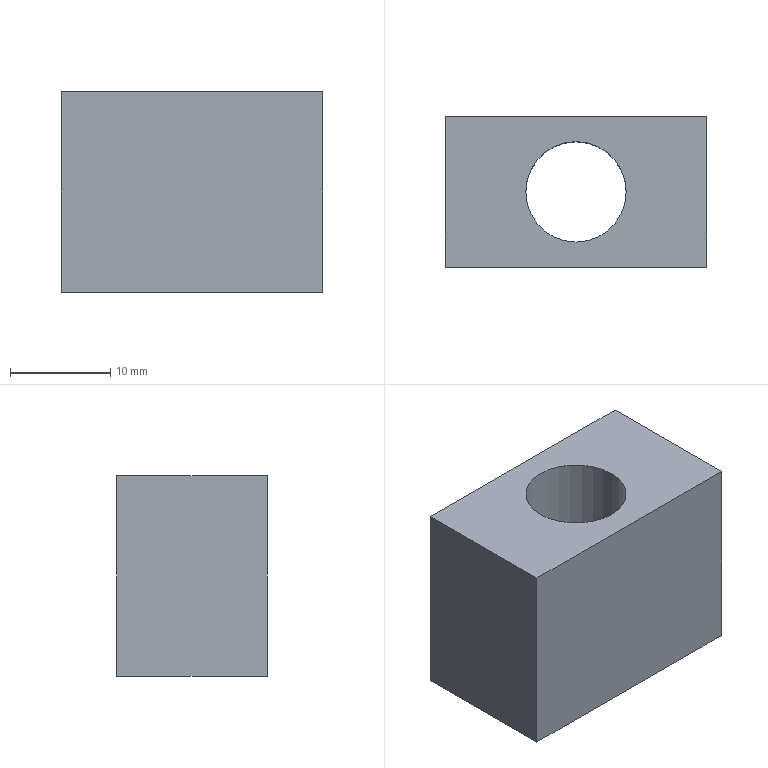Part | SolidWorks | features Extrusion 1 | 1 solid | 8 faces | box 26 x 15 x 20 mm | volume 6229 mm3 | plane 6 | cylinder 2 | commonest cylinder face diameters 10 x2
STEP:
#1=CARTESIAN_POINT('',(-5.,0.,20.));
#2=VERTEX_POINT('',#1);
#3=CARTESIAN_POINT('',(5.,0.,20.));
#4=VERTEX_POINT('',#3);
#5=CARTESIAN_POINT('',(0.,0.,20.));
#6=DIRECTION('',(0.,0.,1.));
#7=DIRECTION('',(1.,0.,0.));
#8=AXIS2_PLACEMENT_3D('',#5,#6,#7);
#9=CIRCLE('',#8,5.);
#10=EDGE_CURVE('',#2,#4,#9,.T.);
#11=ORIENTED_EDGE('',*,*,#10,.T.);
#12=CARTESIAN_POINT('',(5.,0.,0.));
#13=VERTEX_POINT('',#12);
#14=CARTESIAN_POINT('',(5.,0.,20.));
#15=DIRECTION('',(0.,0.,-1.));
#16=VECTOR('',#15,1000.);
#17=LINE('',#14,#16);
#18=EDGE_CURVE('',#4,#13,#17,.T.);
#19=ORIENTED_EDGE('',*,*,#18,.T.);
#20=CARTESIAN_POINT('',(-5.,0.,0.));
#21=VERTEX_POINT('',#20);
#22=CARTESIAN_POINT('',(0.,0.,0.));
#23=DIRECTION('',(0.,0.,1.));
#24=DIRECTION('',(1.,0.,0.));
#25=AXIS2_PLACEMENT_3D('',#22,#23,#24);
#26=CIRCLE('',#25,5.);
#27=EDGE_CURVE('',#21,#13,#26,.T.);
#28=ORIENTED_EDGE('',*,*,#27,.F.);
#29=CARTESIAN_POINT('',(-5.,0.,20.));
#30=DIRECTION('',(0.,0.,-1.));
#31=VECTOR('',#30,1000.);
#32=LINE('',#29,#31);
#33=EDGE_CURVE('',#2,#21,#32,.T.);
#34=ORIENTED_EDGE('',*,*,#33,.F.);
#35=EDGE_LOOP('',(#11,#19,#28,#34));
#36=FACE_OUTER_BOUND('',#35,.T.);
#37=CARTESIAN_POINT('',(0.,0.,20.));
#38=DIRECTION('',(0.,0.,-1.));
#39=DIRECTION('',(-1.,0.,0.));
#40=AXIS2_PLACEMENT_3D('',#37,#38,#39);
#41=CYLINDRICAL_SURFACE('',#40,5.);
#42=ADVANCED_FACE('',(#36),#41,.F.);
#43=CARTESIAN_POINT('',(13.,-7.5,20.));
#44=VERTEX_POINT('',#43);
#45=CARTESIAN_POINT('',(13.,7.5,20.));
#46=VERTEX_POINT('',#45);
#47=CARTESIAN_POINT('',(13.,7.5,20.));
#48=DIRECTION('',(0.,1.,0.));
#49=VECTOR('',#48,1000.);
#50=LINE('',#47,#49);
#51=EDGE_CURVE('',#44,#46,#50,.T.);
#52=ORIENTED_EDGE('',*,*,#51,.T.);
#53=CARTESIAN_POINT('',(-13.,7.5,20.));
#54=VERTEX_POINT('',#53);
#55=CARTESIAN_POINT('',(-13.,7.5,20.));
#56=DIRECTION('',(-1.,0.,0.));
#57=VECTOR('',#56,1000.);
#58=LINE('',#55,#57);
#59=EDGE_CURVE('',#46,#54,#58,.T.);
#60=ORIENTED_EDGE('',*,*,#59,.T.);
#61=CARTESIAN_POINT('',(-13.,-7.5,20.));
#62=VERTEX_POINT('',#61);
#63=CARTESIAN_POINT('',(-13.,7.5,20.));
#64=DIRECTION('',(0.,-1.,0.));
#65=VECTOR('',#64,1000.);
#66=LINE('',#63,#65);
#67=EDGE_CURVE('',#54,#62,#66,.T.);
#68=ORIENTED_EDGE('',*,*,#67,.T.);
#69=CARTESIAN_POINT('',(-13.,-7.5,20.));
#70=DIRECTION('',(1.,0.,0.));
#71=VECTOR('',#70,1000.);
#72=LINE('',#69,#71);
#73=EDGE_CURVE('',#62,#44,#72,.T.);
#74=ORIENTED_EDGE('',*,*,#73,.T.);
#75=EDGE_LOOP('',(#52,#60,#68,#74));
#76=FACE_OUTER_BOUND('',#75,.T.);
#77=ORIENTED_EDGE('',*,*,#10,.F.);
#78=CARTESIAN_POINT('',(0.,0.,20.));
#79=DIRECTION('',(0.,0.,1.));
#80=DIRECTION('',(1.,0.,0.));
#81=AXIS2_PLACEMENT_3D('',#78,#79,#80);
#82=CIRCLE('',#81,5.);
#83=EDGE_CURVE('',#4,#2,#82,.T.);
#84=ORIENTED_EDGE('',*,*,#83,.F.);
#85=EDGE_LOOP('',(#77,#84));
#86=FACE_BOUND('',#85,.T.);
#87=CARTESIAN_POINT('',(0.,0.,20.));
#88=DIRECTION('',(0.,0.,1.));
#89=DIRECTION('',(1.,0.,0.));
#90=AXIS2_PLACEMENT_3D('',#87,#88,#89);
#91=PLANE('',#90);
#92=ADVANCED_FACE('',(#76,#86),#91,.T.);
#93=CARTESIAN_POINT('',(13.,-7.5,0.));
#94=VERTEX_POINT('',#93);
#95=CARTESIAN_POINT('',(13.,7.5,0.));
#96=VERTEX_POINT('',#95);
#97=CARTESIAN_POINT('',(13.,7.5,0.));
#98=DIRECTION('',(0.,1.,0.));
#99=VECTOR('',#98,1000.);
#100=LINE('',#97,#99);
#101=EDGE_CURVE('',#94,#96,#100,.T.);
#102=ORIENTED_EDGE('',*,*,#101,.F.);
#103=CARTESIAN_POINT('',(-13.,-7.5,0.));
#104=VERTEX_POINT('',#103);
#105=CARTESIAN_POINT('',(-13.,-7.5,0.));
#106=DIRECTION('',(1.,0.,0.));
#107=VECTOR('',#106,1000.);
#108=LINE('',#105,#107);
#109=EDGE_CURVE('',#104,#94,#108,.T.);
#110=ORIENTED_EDGE('',*,*,#109,.F.);
#111=CARTESIAN_POINT('',(-13.,7.5,0.));
#112=VERTEX_POINT('',#111);
#113=CARTESIAN_POINT('',(-13.,7.5,0.));
#114=DIRECTION('',(0.,-1.,0.));
#115=VECTOR('',#114,1000.);
#116=LINE('',#113,#115);
#117=EDGE_CURVE('',#112,#104,#116,.T.);
#118=ORIENTED_EDGE('',*,*,#117,.F.);
#119=CARTESIAN_POINT('',(-13.,7.5,0.));
#120=DIRECTION('',(-1.,0.,0.));
#121=VECTOR('',#120,1000.);
#122=LINE('',#119,#121);
#123=EDGE_CURVE('',#96,#112,#122,.T.);
#124=ORIENTED_EDGE('',*,*,#123,.F.);
#125=EDGE_LOOP('',(#102,#110,#118,#124));
#126=FACE_OUTER_BOUND('',#125,.T.);
#127=ORIENTED_EDGE('',*,*,#27,.T.);
#128=CARTESIAN_POINT('',(0.,0.,0.));
#129=DIRECTION('',(0.,0.,1.));
#130=DIRECTION('',(1.,0.,0.));
#131=AXIS2_PLACEMENT_3D('',#128,#129,#130);
#132=CIRCLE('',#131,5.);
#133=EDGE_CURVE('',#13,#21,#132,.T.);
#134=ORIENTED_EDGE('',*,*,#133,.T.);
#135=EDGE_LOOP('',(#127,#134));
#136=FACE_BOUND('',#135,.T.);
#137=CARTESIAN_POINT('',(0.,0.,0.));
#138=DIRECTION('',(0.,0.,1.));
#139=DIRECTION('',(1.,0.,0.));
#140=AXIS2_PLACEMENT_3D('',#137,#138,#139);
#141=PLANE('',#140);
#142=ADVANCED_FACE('',(#126,#136),#141,.F.);
#143=ORIENTED_EDGE('',*,*,#101,.T.);
#144=CARTESIAN_POINT('',(13.,7.5,20.));
#145=DIRECTION('',(0.,0.,-1.));
#146=VECTOR('',#145,1000.);
#147=LINE('',#144,#146);
#148=EDGE_CURVE('',#46,#96,#147,.T.);
#149=ORIENTED_EDGE('',*,*,#148,.F.);
#150=ORIENTED_EDGE('',*,*,#51,.F.);
#151=CARTESIAN_POINT('',(13.,-7.5,20.));
#152=DIRECTION('',(0.,0.,-1.));
#153=VECTOR('',#152,1000.);
#154=LINE('',#151,#153);
#155=EDGE_CURVE('',#44,#94,#154,.T.);
#156=ORIENTED_EDGE('',*,*,#155,.T.);
#157=EDGE_LOOP('',(#143,#149,#150,#156));
#158=FACE_OUTER_BOUND('',#157,.T.);
#159=CARTESIAN_POINT('',(13.,7.5,20.));
#160=DIRECTION('',(-1.,0.,0.));
#161=DIRECTION('',(0.,0.,1.));
#162=AXIS2_PLACEMENT_3D('',#159,#160,#161);
#163=PLANE('',#162);
#164=ADVANCED_FACE('',(#158),#163,.F.);
#165=ORIENTED_EDGE('',*,*,#123,.T.);
#166=CARTESIAN_POINT('',(-13.,7.5,20.));
#167=DIRECTION('',(0.,0.,-1.));
#168=VECTOR('',#167,1000.);
#169=LINE('',#166,#168);
#170=EDGE_CURVE('',#54,#112,#169,.T.);
#171=ORIENTED_EDGE('',*,*,#170,.F.);
#172=ORIENTED_EDGE('',*,*,#59,.F.);
#173=ORIENTED_EDGE('',*,*,#148,.T.);
#174=EDGE_LOOP('',(#165,#171,#172,#173));
#175=FACE_OUTER_BOUND('',#174,.T.);
#176=CARTESIAN_POINT('',(-13.,7.5,20.));
#177=DIRECTION('',(0.,-1.,0.));
#178=DIRECTION('',(0.,0.,-1.));
#179=AXIS2_PLACEMENT_3D('',#176,#177,#178);
#180=PLANE('',#179);
#181=ADVANCED_FACE('',(#175),#180,.F.);
#182=ORIENTED_EDGE('',*,*,#117,.T.);
#183=CARTESIAN_POINT('',(-13.,-7.5,20.));
#184=DIRECTION('',(0.,0.,-1.));
#185=VECTOR('',#184,1000.);
#186=LINE('',#183,#185);
#187=EDGE_CURVE('',#62,#104,#186,.T.);
#188=ORIENTED_EDGE('',*,*,#187,.F.);
#189=ORIENTED_EDGE('',*,*,#67,.F.);
#190=ORIENTED_EDGE('',*,*,#170,.T.);
#191=EDGE_LOOP('',(#182,#188,#189,#190));
#192=FACE_OUTER_BOUND('',#191,.T.);
#193=CARTESIAN_POINT('',(-13.,7.5,20.));
#194=DIRECTION('',(1.,0.,0.));
#195=DIRECTION('',(0.,1.,0.));
#196=AXIS2_PLACEMENT_3D('',#193,#194,#195);
#197=PLANE('',#196);
#198=ADVANCED_FACE('',(#192),#197,.F.);
#199=ORIENTED_EDGE('',*,*,#109,.T.);
#200=ORIENTED_EDGE('',*,*,#155,.F.);
#201=ORIENTED_EDGE('',*,*,#73,.F.);
#202=ORIENTED_EDGE('',*,*,#187,.T.);
#203=EDGE_LOOP('',(#199,#200,#201,#202));
#204=FACE_OUTER_BOUND('',#203,.T.);
#205=CARTESIAN_POINT('',(-13.,-7.5,20.));
#206=DIRECTION('',(0.,1.,0.));
#207=DIRECTION('',(0.,0.,1.));
#208=AXIS2_PLACEMENT_3D('',#205,#206,#207);
#209=PLANE('',#208);
#210=ADVANCED_FACE('',(#204),#209,.F.);
#211=ORIENTED_EDGE('',*,*,#18,.F.);
#212=ORIENTED_EDGE('',*,*,#83,.T.);
#213=ORIENTED_EDGE('',*,*,#33,.T.);
#214=ORIENTED_EDGE('',*,*,#133,.F.);
#215=EDGE_LOOP('',(#211,#212,#213,#214));
#216=FACE_OUTER_BOUND('',#215,.T.);
#217=CARTESIAN_POINT('',(0.,0.,20.));
#218=DIRECTION('',(0.,0.,-1.));
#219=DIRECTION('',(-1.,0.,0.));
#220=AXIS2_PLACEMENT_3D('',#217,#218,#219);
#221=CYLINDRICAL_SURFACE('',#220,5.);
#222=ADVANCED_FACE('',(#216),#221,.F.);
#223=CLOSED_SHELL('',(#42,#92,#142,#164,#181,#198,#210,#222));
#224=MANIFOLD_SOLID_BREP('',#223);
#225=CARTESIAN_POINT('',(0.,0.,0.));
#226=DIRECTION('',(0.,0.,1.));
#227=DIRECTION('',(1.,0.,0.));
#228=AXIS2_PLACEMENT_3D('',#225,#226,#227);
#229=(LENGTH_UNIT()NAMED_UNIT(*)SI_UNIT(.MILLI.,.METRE.));
#230=UNCERTAINTY_MEASURE_WITH_UNIT(LENGTH_MEASURE(0.00001),#229,'','');
#231=(NAMED_UNIT(*)PLANE_ANGLE_UNIT()SI_UNIT($,.RADIAN.));
#232=(NAMED_UNIT(*)SI_UNIT($,.STERADIAN.)SOLID_ANGLE_UNIT());
#233=(GEOMETRIC_REPRESENTATION_CONTEXT(3)GLOBAL_UNCERTAINTY_ASSIGNED_CONTEXT((#230))GLOBAL_UNIT_ASSIGNED_CONTEXT((#229,#231,#232))REPRESENTATION_CONTEXT('',''));
#234=ADVANCED_BREP_SHAPE_REPRESENTATION('',(#224,#228),#233);